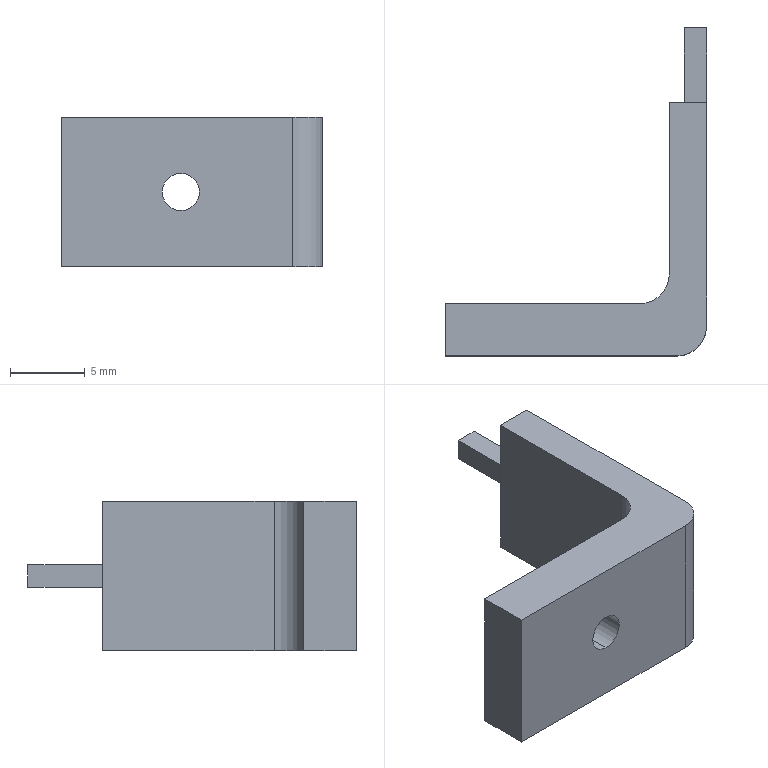Part | SolidWorks | features Extrusion 1, Fillet 1, HoleWzd 1, ICE 1 | 1 solid | 16 faces | box 17.5 x 22 x 10 mm | volume 944.069 mm3 | plane 12 | cylinder 4 | commonest cylinder face diameters 2.5 x2 4 x2
STEP:
#1=CARTESIAN_POINT('',(8.,0.,3.75));
#2=VERTEX_POINT('',#1);
#3=CARTESIAN_POINT('',(8.,0.,6.25));
#4=VERTEX_POINT('',#3);
#5=CARTESIAN_POINT('',(8.,0.,5.));
#6=DIRECTION('',(0.,1.,0.));
#7=DIRECTION('',(0.,0.,1.));
#8=AXIS2_PLACEMENT_3D('',#5,#6,#7);
#9=CIRCLE('',#8,1.25);
#10=EDGE_CURVE('',#2,#4,#9,.T.);
#11=ORIENTED_EDGE('',*,*,#10,.F.);
#12=CARTESIAN_POINT('',(8.,3.5,3.75));
#13=VERTEX_POINT('',#12);
#14=CARTESIAN_POINT('',(8.,3.5,3.75));
#15=DIRECTION('',(0.,1.,0.));
#16=VECTOR('',#15,1000.);
#17=LINE('',#14,#16);
#18=EDGE_CURVE('',#2,#13,#17,.T.);
#19=ORIENTED_EDGE('',*,*,#18,.T.);
#20=CARTESIAN_POINT('',(8.,3.5,6.25));
#21=VERTEX_POINT('',#20);
#22=CARTESIAN_POINT('',(8.,3.5,5.));
#23=DIRECTION('',(0.,1.,0.));
#24=DIRECTION('',(0.,0.,1.));
#25=AXIS2_PLACEMENT_3D('',#22,#23,#24);
#26=CIRCLE('',#25,1.25);
#27=EDGE_CURVE('',#13,#21,#26,.T.);
#28=ORIENTED_EDGE('',*,*,#27,.T.);
#29=CARTESIAN_POINT('',(8.,3.5,6.25));
#30=DIRECTION('',(0.,1.,0.));
#31=VECTOR('',#30,1000.);
#32=LINE('',#29,#31);
#33=EDGE_CURVE('',#4,#21,#32,.T.);
#34=ORIENTED_EDGE('',*,*,#33,.F.);
#35=EDGE_LOOP('',(#11,#19,#28,#34));
#36=FACE_OUTER_BOUND('',#35,.T.);
#37=CARTESIAN_POINT('',(8.,3.5,5.));
#38=DIRECTION('',(0.,1.,0.));
#39=DIRECTION('',(0.,0.,1.));
#40=AXIS2_PLACEMENT_3D('',#37,#38,#39);
#41=CYLINDRICAL_SURFACE('',#40,1.25);
#42=ADVANCED_FACE('',(#36),#41,.F.);
#43=CARTESIAN_POINT('',(16.,17.,5.75));
#44=VERTEX_POINT('',#43);
#45=CARTESIAN_POINT('',(17.5,17.,5.75));
#46=VERTEX_POINT('',#45);
#47=CARTESIAN_POINT('',(16.,17.,5.75));
#48=DIRECTION('',(1.,0.,0.));
#49=VECTOR('',#48,1000.);
#50=LINE('',#47,#49);
#51=EDGE_CURVE('',#44,#46,#50,.T.);
#52=ORIENTED_EDGE('',*,*,#51,.F.);
#53=CARTESIAN_POINT('',(16.,17.,4.25));
#54=VERTEX_POINT('',#53);
#55=CARTESIAN_POINT('',(16.,17.,5.75));
#56=DIRECTION('',(0.,0.,-1.));
#57=VECTOR('',#56,1000.);
#58=LINE('',#55,#57);
#59=EDGE_CURVE('',#44,#54,#58,.T.);
#60=ORIENTED_EDGE('',*,*,#59,.T.);
#61=CARTESIAN_POINT('',(17.5,17.,4.25));
#62=VERTEX_POINT('',#61);
#63=CARTESIAN_POINT('',(16.,17.,4.25));
#64=DIRECTION('',(1.,0.,0.));
#65=VECTOR('',#64,1000.);
#66=LINE('',#63,#65);
#67=EDGE_CURVE('',#54,#62,#66,.T.);
#68=ORIENTED_EDGE('',*,*,#67,.T.);
#69=CARTESIAN_POINT('',(17.5,17.,0.));
#70=VERTEX_POINT('',#69);
#71=CARTESIAN_POINT('',(17.5,17.,10.));
#72=DIRECTION('',(0.,0.,-1.));
#73=VECTOR('',#72,1000.);
#74=LINE('',#71,#73);
#75=EDGE_CURVE('',#62,#70,#74,.T.);
#76=ORIENTED_EDGE('',*,*,#75,.T.);
#77=CARTESIAN_POINT('',(15.,17.,0.));
#78=VERTEX_POINT('',#77);
#79=CARTESIAN_POINT('',(17.5,17.,0.));
#80=DIRECTION('',(-1.,0.,0.));
#81=VECTOR('',#80,1000.);
#82=LINE('',#79,#81);
#83=EDGE_CURVE('',#70,#78,#82,.T.);
#84=ORIENTED_EDGE('',*,*,#83,.T.);
#85=CARTESIAN_POINT('',(15.,17.,10.));
#86=VERTEX_POINT('',#85);
#87=CARTESIAN_POINT('',(15.,17.,10.));
#88=DIRECTION('',(0.,0.,-1.));
#89=VECTOR('',#88,1000.);
#90=LINE('',#87,#89);
#91=EDGE_CURVE('',#86,#78,#90,.T.);
#92=ORIENTED_EDGE('',*,*,#91,.F.);
#93=CARTESIAN_POINT('',(17.5,17.,10.));
#94=VERTEX_POINT('',#93);
#95=CARTESIAN_POINT('',(17.5,17.,10.));
#96=DIRECTION('',(-1.,0.,0.));
#97=VECTOR('',#96,1000.);
#98=LINE('',#95,#97);
#99=EDGE_CURVE('',#94,#86,#98,.T.);
#100=ORIENTED_EDGE('',*,*,#99,.F.);
#101=CARTESIAN_POINT('',(17.5,17.,10.));
#102=DIRECTION('',(0.,0.,-1.));
#103=VECTOR('',#102,1000.);
#104=LINE('',#101,#103);
#105=EDGE_CURVE('',#94,#46,#104,.T.);
#106=ORIENTED_EDGE('',*,*,#105,.T.);
#107=EDGE_LOOP('',(#52,#60,#68,#76,#84,#92,#100,#106));
#108=FACE_OUTER_BOUND('',#107,.T.);
#109=CARTESIAN_POINT('',(17.5,17.,10.));
#110=DIRECTION('',(0.,-1.,0.));
#111=DIRECTION('',(0.,0.,-1.));
#112=AXIS2_PLACEMENT_3D('',#109,#110,#111);
#113=PLANE('',#112);
#114=ADVANCED_FACE('',(#108),#113,.F.);
#115=CARTESIAN_POINT('',(0.,3.5,0.));
#116=VERTEX_POINT('',#115);
#117=CARTESIAN_POINT('',(0.,0.,0.));
#118=VERTEX_POINT('',#117);
#119=CARTESIAN_POINT('',(0.,3.5,0.));
#120=DIRECTION('',(0.,-1.,0.));
#121=VECTOR('',#120,1000.);
#122=LINE('',#119,#121);
#123=EDGE_CURVE('',#116,#118,#122,.T.);
#124=ORIENTED_EDGE('',*,*,#123,.T.);
#125=CARTESIAN_POINT('',(0.,0.,10.));
#126=VERTEX_POINT('',#125);
#127=CARTESIAN_POINT('',(0.,0.,10.));
#128=DIRECTION('',(0.,0.,-1.));
#129=VECTOR('',#128,1000.);
#130=LINE('',#127,#129);
#131=EDGE_CURVE('',#126,#118,#130,.T.);
#132=ORIENTED_EDGE('',*,*,#131,.F.);
#133=CARTESIAN_POINT('',(0.,3.5,10.));
#134=VERTEX_POINT('',#133);
#135=CARTESIAN_POINT('',(0.,3.5,10.));
#136=DIRECTION('',(0.,-1.,0.));
#137=VECTOR('',#136,1000.);
#138=LINE('',#135,#137);
#139=EDGE_CURVE('',#134,#126,#138,.T.);
#140=ORIENTED_EDGE('',*,*,#139,.F.);
#141=CARTESIAN_POINT('',(0.,3.5,10.));
#142=DIRECTION('',(0.,0.,-1.));
#143=VECTOR('',#142,1000.);
#144=LINE('',#141,#143);
#145=EDGE_CURVE('',#134,#116,#144,.T.);
#146=ORIENTED_EDGE('',*,*,#145,.T.);
#147=EDGE_LOOP('',(#124,#132,#140,#146));
#148=FACE_OUTER_BOUND('',#147,.T.);
#149=CARTESIAN_POINT('',(0.,3.5,10.));
#150=DIRECTION('',(1.,0.,0.));
#151=DIRECTION('',(0.,1.,0.));
#152=AXIS2_PLACEMENT_3D('',#149,#150,#151);
#153=PLANE('',#152);
#154=ADVANCED_FACE('',(#148),#153,.F.);
#155=CARTESIAN_POINT('',(8.,0.,5.));
#156=DIRECTION('',(0.,1.,0.));
#157=DIRECTION('',(0.,0.,1.));
#158=AXIS2_PLACEMENT_3D('',#155,#156,#157);
#159=CIRCLE('',#158,1.25);
#160=EDGE_CURVE('',#4,#2,#159,.T.);
#161=ORIENTED_EDGE('',*,*,#160,.T.);
#162=ORIENTED_EDGE('',*,*,#10,.T.);
#163=EDGE_LOOP('',(#161,#162));
#164=FACE_BOUND('',#163,.T.);
#165=CARTESIAN_POINT('',(15.5,0.,0.));
#166=VERTEX_POINT('',#165);
#167=CARTESIAN_POINT('',(0.,0.,0.));
#168=DIRECTION('',(1.,0.,0.));
#169=VECTOR('',#168,1000.);
#170=LINE('',#167,#169);
#171=EDGE_CURVE('',#118,#166,#170,.T.);
#172=ORIENTED_EDGE('',*,*,#171,.T.);
#173=CARTESIAN_POINT('',(15.5,0.,10.));
#174=VERTEX_POINT('',#173);
#175=CARTESIAN_POINT('',(15.5,0.,10.));
#176=DIRECTION('',(0.,0.,1.));
#177=VECTOR('',#176,1000.);
#178=LINE('',#175,#177);
#179=EDGE_CURVE('',#166,#174,#178,.T.);
#180=ORIENTED_EDGE('',*,*,#179,.T.);
#181=CARTESIAN_POINT('',(0.,0.,10.));
#182=DIRECTION('',(1.,0.,0.));
#183=VECTOR('',#182,1000.);
#184=LINE('',#181,#183);
#185=EDGE_CURVE('',#126,#174,#184,.T.);
#186=ORIENTED_EDGE('',*,*,#185,.F.);
#187=ORIENTED_EDGE('',*,*,#131,.T.);
#188=EDGE_LOOP('',(#172,#180,#186,#187));
#189=FACE_OUTER_BOUND('',#188,.T.);
#190=CARTESIAN_POINT('',(0.,0.,10.));
#191=DIRECTION('',(0.,1.,0.));
#192=DIRECTION('',(0.,0.,1.));
#193=AXIS2_PLACEMENT_3D('',#190,#191,#192);
#194=PLANE('',#193);
#195=ADVANCED_FACE('',(#164,#189),#194,.F.);
#196=CARTESIAN_POINT('',(17.5,2.,10.));
#197=VERTEX_POINT('',#196);
#198=CARTESIAN_POINT('',(17.5,0.,10.));
#199=DIRECTION('',(0.,1.,0.));
#200=VECTOR('',#199,1000.);
#201=LINE('',#198,#200);
#202=EDGE_CURVE('',#197,#94,#201,.T.);
#203=ORIENTED_EDGE('',*,*,#202,.F.);
#204=CARTESIAN_POINT('',(17.5,2.,0.));
#205=VERTEX_POINT('',#204);
#206=CARTESIAN_POINT('',(17.5,2.,10.));
#207=DIRECTION('',(0.,0.,-1.));
#208=VECTOR('',#207,1000.);
#209=LINE('',#206,#208);
#210=EDGE_CURVE('',#197,#205,#209,.T.);
#211=ORIENTED_EDGE('',*,*,#210,.T.);
#212=CARTESIAN_POINT('',(17.5,0.,0.));
#213=DIRECTION('',(0.,1.,0.));
#214=VECTOR('',#213,1000.);
#215=LINE('',#212,#214);
#216=EDGE_CURVE('',#205,#70,#215,.T.);
#217=ORIENTED_EDGE('',*,*,#216,.T.);
#218=ORIENTED_EDGE('',*,*,#75,.F.);
#219=CARTESIAN_POINT('',(17.5,22.,4.25));
#220=VERTEX_POINT('',#219);
#221=CARTESIAN_POINT('',(17.5,22.,4.25));
#222=DIRECTION('',(0.,1.,0.));
#223=VECTOR('',#222,1000.);
#224=LINE('',#221,#223);
#225=EDGE_CURVE('',#62,#220,#224,.T.);
#226=ORIENTED_EDGE('',*,*,#225,.T.);
#227=CARTESIAN_POINT('',(17.5,22.,5.75));
#228=VERTEX_POINT('',#227);
#229=CARTESIAN_POINT('',(17.5,22.,5.75));
#230=DIRECTION('',(0.,0.,1.));
#231=VECTOR('',#230,1000.);
#232=LINE('',#229,#231);
#233=EDGE_CURVE('',#220,#228,#232,.T.);
#234=ORIENTED_EDGE('',*,*,#233,.T.);
#235=CARTESIAN_POINT('',(17.5,17.,5.75));
#236=DIRECTION('',(0.,-1.,0.));
#237=VECTOR('',#236,1000.);
#238=LINE('',#235,#237);
#239=EDGE_CURVE('',#228,#46,#238,.T.);
#240=ORIENTED_EDGE('',*,*,#239,.T.);
#241=ORIENTED_EDGE('',*,*,#105,.F.);
#242=EDGE_LOOP('',(#203,#211,#217,#218,#226,#234,#240,#241));
#243=FACE_OUTER_BOUND('',#242,.T.);
#244=CARTESIAN_POINT('',(17.5,0.,10.));
#245=DIRECTION('',(-1.,0.,0.));
#246=DIRECTION('',(0.,0.,1.));
#247=AXIS2_PLACEMENT_3D('',#244,#245,#246);
#248=PLANE('',#247);
#249=ADVANCED_FACE('',(#243),#248,.F.);
#250=CARTESIAN_POINT('',(15.,5.5,0.));
#251=VERTEX_POINT('',#250);
#252=CARTESIAN_POINT('',(15.,17.,0.));
#253=DIRECTION('',(0.,-1.,0.));
#254=VECTOR('',#253,1000.);
#255=LINE('',#252,#254);
#256=EDGE_CURVE('',#78,#251,#255,.T.);
#257=ORIENTED_EDGE('',*,*,#256,.T.);
#258=CARTESIAN_POINT('',(15.,5.5,10.));
#259=VERTEX_POINT('',#258);
#260=CARTESIAN_POINT('',(15.,5.5,10.));
#261=DIRECTION('',(0.,0.,1.));
#262=VECTOR('',#261,1000.);
#263=LINE('',#260,#262);
#264=EDGE_CURVE('',#251,#259,#263,.T.);
#265=ORIENTED_EDGE('',*,*,#264,.T.);
#266=CARTESIAN_POINT('',(15.,17.,10.));
#267=DIRECTION('',(0.,-1.,0.));
#268=VECTOR('',#267,1000.);
#269=LINE('',#266,#268);
#270=EDGE_CURVE('',#86,#259,#269,.T.);
#271=ORIENTED_EDGE('',*,*,#270,.F.);
#272=ORIENTED_EDGE('',*,*,#91,.T.);
#273=EDGE_LOOP('',(#257,#265,#271,#272));
#274=FACE_OUTER_BOUND('',#273,.T.);
#275=CARTESIAN_POINT('',(15.,17.,10.));
#276=DIRECTION('',(1.,0.,0.));
#277=DIRECTION('',(0.,1.,0.));
#278=AXIS2_PLACEMENT_3D('',#275,#276,#277);
#279=PLANE('',#278);
#280=ADVANCED_FACE('',(#274),#279,.F.);
#281=CARTESIAN_POINT('',(8.,3.5,5.));
#282=DIRECTION('',(0.,1.,0.));
#283=DIRECTION('',(0.,0.,1.));
#284=AXIS2_PLACEMENT_3D('',#281,#282,#283);
#285=CIRCLE('',#284,1.25);
#286=EDGE_CURVE('',#21,#13,#285,.T.);
#287=ORIENTED_EDGE('',*,*,#286,.F.);
#288=ORIENTED_EDGE('',*,*,#27,.F.);
#289=EDGE_LOOP('',(#287,#288));
#290=FACE_BOUND('',#289,.T.);
#291=CARTESIAN_POINT('',(13.,3.5,10.));
#292=VERTEX_POINT('',#291);
#293=CARTESIAN_POINT('',(15.,3.5,10.));
#294=DIRECTION('',(-1.,0.,0.));
#295=VECTOR('',#294,1000.);
#296=LINE('',#293,#295);
#297=EDGE_CURVE('',#292,#134,#296,.T.);
#298=ORIENTED_EDGE('',*,*,#297,.F.);
#299=CARTESIAN_POINT('',(13.,3.5,0.));
#300=VERTEX_POINT('',#299);
#301=CARTESIAN_POINT('',(13.,3.5,0.));
#302=DIRECTION('',(0.,0.,-1.));
#303=VECTOR('',#302,1000.);
#304=LINE('',#301,#303);
#305=EDGE_CURVE('',#292,#300,#304,.T.);
#306=ORIENTED_EDGE('',*,*,#305,.T.);
#307=CARTESIAN_POINT('',(15.,3.5,0.));
#308=DIRECTION('',(-1.,0.,0.));
#309=VECTOR('',#308,1000.);
#310=LINE('',#307,#309);
#311=EDGE_CURVE('',#300,#116,#310,.T.);
#312=ORIENTED_EDGE('',*,*,#311,.T.);
#313=ORIENTED_EDGE('',*,*,#145,.F.);
#314=EDGE_LOOP('',(#298,#306,#312,#313));
#315=FACE_OUTER_BOUND('',#314,.T.);
#316=CARTESIAN_POINT('',(15.,3.5,10.));
#317=DIRECTION('',(0.,-1.,0.));
#318=DIRECTION('',(1.,0.,0.));
#319=AXIS2_PLACEMENT_3D('',#316,#317,#318);
#320=PLANE('',#319);
#321=ADVANCED_FACE('',(#290,#315),#320,.F.);
#322=ORIENTED_EDGE('',*,*,#185,.T.);
#323=CARTESIAN_POINT('',(15.5,2.,10.));
#324=DIRECTION('',(0.,0.,1.));
#325=DIRECTION('',(1.,0.,0.));
#326=AXIS2_PLACEMENT_3D('',#323,#324,#325);
#327=CIRCLE('',#326,2.);
#328=EDGE_CURVE('',#174,#197,#327,.T.);
#329=ORIENTED_EDGE('',*,*,#328,.T.);
#330=ORIENTED_EDGE('',*,*,#202,.T.);
#331=ORIENTED_EDGE('',*,*,#99,.T.);
#332=ORIENTED_EDGE('',*,*,#270,.T.);
#333=CARTESIAN_POINT('',(13.,5.5,10.));
#334=DIRECTION('',(0.,0.,-1.));
#335=DIRECTION('',(1.,0.,0.));
#336=AXIS2_PLACEMENT_3D('',#333,#334,#335);
#337=CIRCLE('',#336,2.);
#338=EDGE_CURVE('',#259,#292,#337,.T.);
#339=ORIENTED_EDGE('',*,*,#338,.T.);
#340=ORIENTED_EDGE('',*,*,#297,.T.);
#341=ORIENTED_EDGE('',*,*,#139,.T.);
#342=EDGE_LOOP('',(#322,#329,#330,#331,#332,#339,#340,#341));
#343=FACE_OUTER_BOUND('',#342,.T.);
#344=CARTESIAN_POINT('',(0.,0.,10.));
#345=DIRECTION('',(0.,0.,1.));
#346=DIRECTION('',(1.,0.,0.));
#347=AXIS2_PLACEMENT_3D('',#344,#345,#346);
#348=PLANE('',#347);
#349=ADVANCED_FACE('',(#343),#348,.T.);
#350=ORIENTED_EDGE('',*,*,#216,.F.);
#351=CARTESIAN_POINT('',(15.5,2.,0.));
#352=DIRECTION('',(0.,0.,-1.));
#353=DIRECTION('',(1.,0.,0.));
#354=AXIS2_PLACEMENT_3D('',#351,#352,#353);
#355=CIRCLE('',#354,2.);
#356=EDGE_CURVE('',#205,#166,#355,.T.);
#357=ORIENTED_EDGE('',*,*,#356,.T.);
#358=ORIENTED_EDGE('',*,*,#171,.F.);
#359=ORIENTED_EDGE('',*,*,#123,.F.);
#360=ORIENTED_EDGE('',*,*,#311,.F.);
#361=CARTESIAN_POINT('',(13.,5.5,0.));
#362=DIRECTION('',(0.,0.,1.));
#363=DIRECTION('',(1.,0.,0.));
#364=AXIS2_PLACEMENT_3D('',#361,#362,#363);
#365=CIRCLE('',#364,2.);
#366=EDGE_CURVE('',#300,#251,#365,.T.);
#367=ORIENTED_EDGE('',*,*,#366,.T.);
#368=ORIENTED_EDGE('',*,*,#256,.F.);
#369=ORIENTED_EDGE('',*,*,#83,.F.);
#370=EDGE_LOOP('',(#350,#357,#358,#359,#360,#367,#368,#369));
#371=FACE_OUTER_BOUND('',#370,.T.);
#372=CARTESIAN_POINT('',(0.,0.,0.));
#373=DIRECTION('',(0.,0.,1.));
#374=DIRECTION('',(1.,0.,0.));
#375=AXIS2_PLACEMENT_3D('',#372,#373,#374);
#376=PLANE('',#375);
#377=ADVANCED_FACE('',(#371),#376,.F.);
#378=ORIENTED_EDGE('',*,*,#239,.F.);
#379=CARTESIAN_POINT('',(16.,22.,5.75));
#380=VERTEX_POINT('',#379);
#381=CARTESIAN_POINT('',(16.,22.,5.75));
#382=DIRECTION('',(1.,0.,0.));
#383=VECTOR('',#382,1000.);
#384=LINE('',#381,#383);
#385=EDGE_CURVE('',#380,#228,#384,.T.);
#386=ORIENTED_EDGE('',*,*,#385,.F.);
#387=CARTESIAN_POINT('',(16.,17.,5.75));
#388=DIRECTION('',(0.,-1.,0.));
#389=VECTOR('',#388,1000.);
#390=LINE('',#387,#389);
#391=EDGE_CURVE('',#380,#44,#390,.T.);
#392=ORIENTED_EDGE('',*,*,#391,.T.);
#393=ORIENTED_EDGE('',*,*,#51,.T.);
#394=EDGE_LOOP('',(#378,#386,#392,#393));
#395=FACE_OUTER_BOUND('',#394,.T.);
#396=CARTESIAN_POINT('',(16.,17.,5.75));
#397=DIRECTION('',(0.,0.,1.));
#398=DIRECTION('',(0.,-1.,0.));
#399=AXIS2_PLACEMENT_3D('',#396,#397,#398);
#400=PLANE('',#399);
#401=ADVANCED_FACE('',(#395),#400,.T.);
#402=ORIENTED_EDGE('',*,*,#233,.F.);
#403=CARTESIAN_POINT('',(16.,22.,4.25));
#404=VERTEX_POINT('',#403);
#405=CARTESIAN_POINT('',(16.,22.,4.25));
#406=DIRECTION('',(1.,0.,0.));
#407=VECTOR('',#406,1000.);
#408=LINE('',#405,#407);
#409=EDGE_CURVE('',#404,#220,#408,.T.);
#410=ORIENTED_EDGE('',*,*,#409,.F.);
#411=CARTESIAN_POINT('',(16.,22.,5.75));
#412=DIRECTION('',(0.,0.,1.));
#413=VECTOR('',#412,1000.);
#414=LINE('',#411,#413);
#415=EDGE_CURVE('',#404,#380,#414,.T.);
#416=ORIENTED_EDGE('',*,*,#415,.T.);
#417=ORIENTED_EDGE('',*,*,#385,.T.);
#418=EDGE_LOOP('',(#402,#410,#416,#417));
#419=FACE_OUTER_BOUND('',#418,.T.);
#420=CARTESIAN_POINT('',(16.,22.,5.75));
#421=DIRECTION('',(0.,1.,0.));
#422=DIRECTION('',(0.,0.,1.));
#423=AXIS2_PLACEMENT_3D('',#420,#421,#422);
#424=PLANE('',#423);
#425=ADVANCED_FACE('',(#419),#424,.T.);
#426=ORIENTED_EDGE('',*,*,#225,.F.);
#427=ORIENTED_EDGE('',*,*,#67,.F.);
#428=CARTESIAN_POINT('',(16.,22.,4.25));
#429=DIRECTION('',(0.,1.,0.));
#430=VECTOR('',#429,1000.);
#431=LINE('',#428,#430);
#432=EDGE_CURVE('',#54,#404,#431,.T.);
#433=ORIENTED_EDGE('',*,*,#432,.T.);
#434=ORIENTED_EDGE('',*,*,#409,.T.);
#435=EDGE_LOOP('',(#426,#427,#433,#434));
#436=FACE_OUTER_BOUND('',#435,.T.);
#437=CARTESIAN_POINT('',(16.,22.,4.25));
#438=DIRECTION('',(0.,0.,-1.));
#439=DIRECTION('',(0.,1.,0.));
#440=AXIS2_PLACEMENT_3D('',#437,#438,#439);
#441=PLANE('',#440);
#442=ADVANCED_FACE('',(#436),#441,.T.);
#443=ORIENTED_EDGE('',*,*,#59,.F.);
#444=ORIENTED_EDGE('',*,*,#391,.F.);
#445=ORIENTED_EDGE('',*,*,#415,.F.);
#446=ORIENTED_EDGE('',*,*,#432,.F.);
#447=EDGE_LOOP('',(#443,#444,#445,#446));
#448=FACE_OUTER_BOUND('',#447,.T.);
#449=CARTESIAN_POINT('',(16.,0.,0.));
#450=DIRECTION('',(-1.,0.,0.));
#451=DIRECTION('',(0.,0.,1.));
#452=AXIS2_PLACEMENT_3D('',#449,#450,#451);
#453=PLANE('',#452);
#454=ADVANCED_FACE('',(#448),#453,.T.);
#455=ORIENTED_EDGE('',*,*,#328,.F.);
#456=ORIENTED_EDGE('',*,*,#179,.F.);
#457=ORIENTED_EDGE('',*,*,#356,.F.);
#458=ORIENTED_EDGE('',*,*,#210,.F.);
#459=EDGE_LOOP('',(#455,#456,#457,#458));
#460=FACE_OUTER_BOUND('',#459,.T.);
#461=CARTESIAN_POINT('',(15.5,2.,10.));
#462=DIRECTION('',(0.,0.,-1.));
#463=DIRECTION('',(-1.,0.,0.));
#464=AXIS2_PLACEMENT_3D('',#461,#462,#463);
#465=CYLINDRICAL_SURFACE('',#464,2.);
#466=ADVANCED_FACE('',(#460),#465,.T.);
#467=ORIENTED_EDGE('',*,*,#338,.F.);
#468=ORIENTED_EDGE('',*,*,#264,.F.);
#469=ORIENTED_EDGE('',*,*,#366,.F.);
#470=ORIENTED_EDGE('',*,*,#305,.F.);
#471=EDGE_LOOP('',(#467,#468,#469,#470));
#472=FACE_OUTER_BOUND('',#471,.T.);
#473=CARTESIAN_POINT('',(13.,5.5,10.));
#474=DIRECTION('',(0.,0.,1.));
#475=DIRECTION('',(1.,0.,0.));
#476=AXIS2_PLACEMENT_3D('',#473,#474,#475);
#477=CYLINDRICAL_SURFACE('',#476,2.);
#478=ADVANCED_FACE('',(#472),#477,.F.);
#479=ORIENTED_EDGE('',*,*,#18,.F.);
#480=ORIENTED_EDGE('',*,*,#160,.F.);
#481=ORIENTED_EDGE('',*,*,#33,.T.);
#482=ORIENTED_EDGE('',*,*,#286,.T.);
#483=EDGE_LOOP('',(#479,#480,#481,#482));
#484=FACE_OUTER_BOUND('',#483,.T.);
#485=CARTESIAN_POINT('',(8.,3.5,5.));
#486=DIRECTION('',(0.,1.,0.));
#487=DIRECTION('',(0.,0.,1.));
#488=AXIS2_PLACEMENT_3D('',#485,#486,#487);
#489=CYLINDRICAL_SURFACE('',#488,1.25);
#490=ADVANCED_FACE('',(#484),#489,.F.);
#491=CLOSED_SHELL('',(#42,#114,#154,#195,#249,#280,#321,#349,#377,#401,#425,#442,#454,#466,#478,#490));
#492=MANIFOLD_SOLID_BREP('',#491);
#493=CARTESIAN_POINT('',(0.,0.,0.));
#494=DIRECTION('',(0.,0.,1.));
#495=DIRECTION('',(1.,0.,0.));
#496=AXIS2_PLACEMENT_3D('',#493,#494,#495);
#497=(LENGTH_UNIT()NAMED_UNIT(*)SI_UNIT(.MILLI.,.METRE.));
#498=UNCERTAINTY_MEASURE_WITH_UNIT(LENGTH_MEASURE(0.00001),#497,'','');
#499=(NAMED_UNIT(*)PLANE_ANGLE_UNIT()SI_UNIT($,.RADIAN.));
#500=(NAMED_UNIT(*)SI_UNIT($,.STERADIAN.)SOLID_ANGLE_UNIT());
#501=(GEOMETRIC_REPRESENTATION_CONTEXT(3)GLOBAL_UNCERTAINTY_ASSIGNED_CONTEXT((#498))GLOBAL_UNIT_ASSIGNED_CONTEXT((#497,#499,#500))REPRESENTATION_CONTEXT('',''));
#502=ADVANCED_BREP_SHAPE_REPRESENTATION('',(#492,#496),#501);